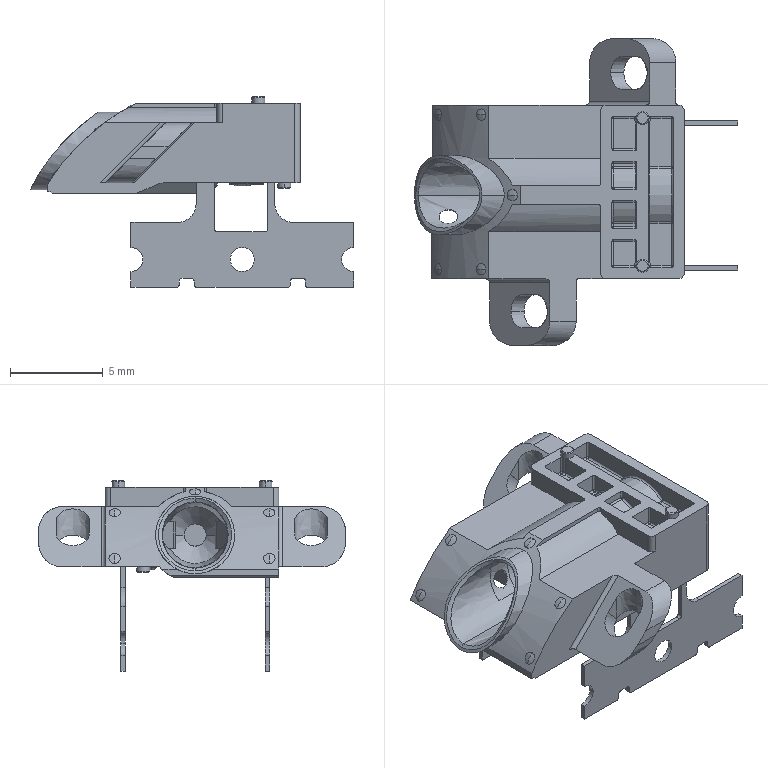Part | NX | 3 solids | 913 faces | box 17.419 x 16.558 x 10.278 mm | volume 312.951 mm3 | plane 478 | cylinder 293 | torus 54 | sphere 48 | spline 22 | cone 18 | commonest cylinder face diameters 0.2 x110 0.3 x32 0.4 x20 0.7 x18 1 x16 1.3 x12